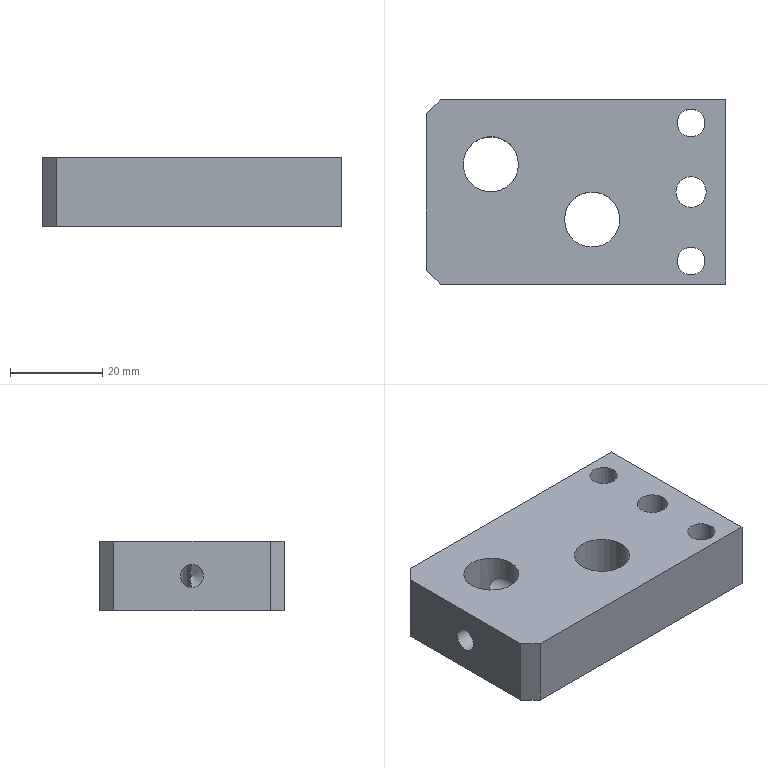Part | NX | features BREP 1 | 1 solid | 20 faces | box 65 x 40 x 15 mm | volume 33188 mm3 | plane 9 | cylinder 9 | cone 2 | commonest cylinder face diameters 5 x3 6 x2 12 x2 6.6 x1 11 x1
STEP:
#1=CARTESIAN_POINT('',(32.5,-20.,0.));
#2=VERTEX_POINT('',#1);
#3=CARTESIAN_POINT('',(32.5,20.,0.));
#4=VERTEX_POINT('',#3);
#5=CARTESIAN_POINT('',(32.5,20.,0.));
#6=DIRECTION('',(0.,1.,0.));
#7=VECTOR('',#6,1000.);
#8=LINE('',#5,#7);
#9=EDGE_CURVE('',#2,#4,#8,.T.);
#10=ORIENTED_EDGE('',*,*,#9,.T.);
#11=CARTESIAN_POINT('',(32.5,20.,15.));
#12=VERTEX_POINT('',#11);
#13=CARTESIAN_POINT('',(32.5,20.,15.));
#14=DIRECTION('',(0.,0.,-1.));
#15=VECTOR('',#14,1000.);
#16=LINE('',#13,#15);
#17=EDGE_CURVE('',#12,#4,#16,.T.);
#18=ORIENTED_EDGE('',*,*,#17,.F.);
#19=CARTESIAN_POINT('',(32.5,-20.,15.));
#20=VERTEX_POINT('',#19);
#21=CARTESIAN_POINT('',(32.5,20.,15.));
#22=DIRECTION('',(0.,1.,0.));
#23=VECTOR('',#22,1000.);
#24=LINE('',#21,#23);
#25=EDGE_CURVE('',#20,#12,#24,.T.);
#26=ORIENTED_EDGE('',*,*,#25,.F.);
#27=CARTESIAN_POINT('',(32.5,-20.,15.));
#28=DIRECTION('',(0.,0.,-1.));
#29=VECTOR('',#28,1000.);
#30=LINE('',#27,#29);
#31=EDGE_CURVE('',#20,#2,#30,.T.);
#32=ORIENTED_EDGE('',*,*,#31,.T.);
#33=EDGE_LOOP('',(#10,#18,#26,#32));
#34=FACE_BOUND('',#33,.T.);
#35=CARTESIAN_POINT('',(32.5,20.,15.));
#36=DIRECTION('',(-1.,0.,0.));
#37=DIRECTION('',(0.,0.,-1.));
#38=AXIS2_PLACEMENT_3D('',#35,#36,#37);
#39=PLANE('',#38);
#40=ADVANCED_FACE('',(#34),#39,.F.);
#41=CARTESIAN_POINT('',(-12.,20.,10.));
#42=VERTEX_POINT('',#41);
#43=CARTESIAN_POINT('',(-12.,20.,7.5));
#44=DIRECTION('',(0.,1.,0.));
#45=DIRECTION('',(0.,0.,1.));
#46=AXIS2_PLACEMENT_3D('',#43,#44,#45);
#47=CIRCLE('',#46,2.5);
#48=EDGE_CURVE('',#42,#42,#47,.T.);
#49=ORIENTED_EDGE('',*,*,#48,.F.);
#50=EDGE_LOOP('',(#49));
#51=FACE_BOUND('',#50,.T.);
#52=CARTESIAN_POINT('',(-29.5,20.,0.));
#53=VERTEX_POINT('',#52);
#54=CARTESIAN_POINT('',(-32.5,20.,0.));
#55=DIRECTION('',(-1.,0.,0.));
#56=VECTOR('',#55,1000.);
#57=LINE('',#54,#56);
#58=EDGE_CURVE('',#4,#53,#57,.T.);
#59=ORIENTED_EDGE('',*,*,#58,.T.);
#60=CARTESIAN_POINT('',(-29.5,20.,15.));
#61=VERTEX_POINT('',#60);
#62=CARTESIAN_POINT('',(-29.5,20.,15.));
#63=DIRECTION('',(0.,0.,1.));
#64=VECTOR('',#63,1000.);
#65=LINE('',#62,#64);
#66=EDGE_CURVE('',#53,#61,#65,.T.);
#67=ORIENTED_EDGE('',*,*,#66,.T.);
#68=CARTESIAN_POINT('',(-32.5,20.,15.));
#69=DIRECTION('',(-1.,0.,0.));
#70=VECTOR('',#69,1000.);
#71=LINE('',#68,#70);
#72=EDGE_CURVE('',#12,#61,#71,.T.);
#73=ORIENTED_EDGE('',*,*,#72,.F.);
#74=ORIENTED_EDGE('',*,*,#17,.T.);
#75=EDGE_LOOP('',(#59,#67,#73,#74));
#76=FACE_BOUND('',#75,.T.);
#77=CARTESIAN_POINT('',(-32.5,20.,15.));
#78=DIRECTION('',(0.,-1.,0.));
#79=DIRECTION('',(0.,0.,1.));
#80=AXIS2_PLACEMENT_3D('',#77,#78,#79);
#81=PLANE('',#80);
#82=ADVANCED_FACE('',(#51,#76),#81,.F.);
#83=CARTESIAN_POINT('',(-32.5,0.,10.));
#84=VERTEX_POINT('',#83);
#85=CARTESIAN_POINT('',(-32.5,0.,7.5));
#86=DIRECTION('',(-1.,0.,0.));
#87=DIRECTION('',(0.,0.,1.));
#88=AXIS2_PLACEMENT_3D('',#85,#86,#87);
#89=CIRCLE('',#88,2.5);
#90=EDGE_CURVE('',#84,#84,#89,.T.);
#91=ORIENTED_EDGE('',*,*,#90,.F.);
#92=EDGE_LOOP('',(#91));
#93=FACE_BOUND('',#92,.T.);
#94=CARTESIAN_POINT('',(-32.5,17.,15.));
#95=VERTEX_POINT('',#94);
#96=CARTESIAN_POINT('',(-32.5,-17.,15.));
#97=VERTEX_POINT('',#96);
#98=CARTESIAN_POINT('',(-32.5,20.,15.));
#99=DIRECTION('',(0.,-1.,0.));
#100=VECTOR('',#99,1000.);
#101=LINE('',#98,#100);
#102=EDGE_CURVE('',#95,#97,#101,.T.);
#103=ORIENTED_EDGE('',*,*,#102,.F.);
#104=CARTESIAN_POINT('',(-32.5,17.,0.));
#105=VERTEX_POINT('',#104);
#106=CARTESIAN_POINT('',(-32.5,17.,15.));
#107=DIRECTION('',(0.,0.,-1.));
#108=VECTOR('',#107,1000.);
#109=LINE('',#106,#108);
#110=EDGE_CURVE('',#95,#105,#109,.T.);
#111=ORIENTED_EDGE('',*,*,#110,.T.);
#112=CARTESIAN_POINT('',(-32.5,-17.,0.));
#113=VERTEX_POINT('',#112);
#114=CARTESIAN_POINT('',(-32.5,20.,0.));
#115=DIRECTION('',(0.,-1.,0.));
#116=VECTOR('',#115,1000.);
#117=LINE('',#114,#116);
#118=EDGE_CURVE('',#105,#113,#117,.T.);
#119=ORIENTED_EDGE('',*,*,#118,.T.);
#120=CARTESIAN_POINT('',(-32.5,-17.,15.));
#121=DIRECTION('',(0.,0.,1.));
#122=VECTOR('',#121,1000.);
#123=LINE('',#120,#122);
#124=EDGE_CURVE('',#113,#97,#123,.T.);
#125=ORIENTED_EDGE('',*,*,#124,.T.);
#126=EDGE_LOOP('',(#103,#111,#119,#125));
#127=FACE_BOUND('',#126,.T.);
#128=CARTESIAN_POINT('',(-32.5,20.,15.));
#129=DIRECTION('',(1.,0.,0.));
#130=DIRECTION('',(0.,-1.,0.));
#131=AXIS2_PLACEMENT_3D('',#128,#129,#130);
#132=PLANE('',#131);
#133=ADVANCED_FACE('',(#93,#127),#132,.F.);
#134=CARTESIAN_POINT('',(-29.5,-20.,15.));
#135=VERTEX_POINT('',#134);
#136=CARTESIAN_POINT('',(-32.5,-20.,15.));
#137=DIRECTION('',(1.,0.,0.));
#138=VECTOR('',#137,1000.);
#139=LINE('',#136,#138);
#140=EDGE_CURVE('',#135,#20,#139,.T.);
#141=ORIENTED_EDGE('',*,*,#140,.F.);
#142=CARTESIAN_POINT('',(-29.5,-20.,0.));
#143=VERTEX_POINT('',#142);
#144=CARTESIAN_POINT('',(-29.5,-20.,15.));
#145=DIRECTION('',(0.,0.,-1.));
#146=VECTOR('',#145,1000.);
#147=LINE('',#144,#146);
#148=EDGE_CURVE('',#135,#143,#147,.T.);
#149=ORIENTED_EDGE('',*,*,#148,.T.);
#150=CARTESIAN_POINT('',(-32.5,-20.,0.));
#151=DIRECTION('',(1.,0.,0.));
#152=VECTOR('',#151,1000.);
#153=LINE('',#150,#152);
#154=EDGE_CURVE('',#143,#2,#153,.T.);
#155=ORIENTED_EDGE('',*,*,#154,.T.);
#156=ORIENTED_EDGE('',*,*,#31,.F.);
#157=EDGE_LOOP('',(#141,#149,#155,#156));
#158=FACE_BOUND('',#157,.T.);
#159=CARTESIAN_POINT('',(-32.5,-20.,15.));
#160=DIRECTION('',(0.,1.,0.));
#161=DIRECTION('',(0.,0.,-1.));
#162=AXIS2_PLACEMENT_3D('',#159,#160,#161);
#163=PLANE('',#162);
#164=ADVANCED_FACE('',(#158),#163,.F.);
#165=CARTESIAN_POINT('',(21.7,0.,15.));
#166=VERTEX_POINT('',#165);
#167=CARTESIAN_POINT('',(25.,0.,15.));
#168=DIRECTION('',(0.,0.,-1.));
#169=DIRECTION('',(-1.,0.,0.));
#170=AXIS2_PLACEMENT_3D('',#167,#168,#169);
#171=CIRCLE('',#170,3.3);
#172=EDGE_CURVE('',#166,#166,#171,.T.);
#173=ORIENTED_EDGE('',*,*,#172,.T.);
#174=EDGE_LOOP('',(#173));
#175=FACE_BOUND('',#174,.T.);
#176=CARTESIAN_POINT('',(28.,-15.,15.));
#177=VERTEX_POINT('',#176);
#178=CARTESIAN_POINT('',(25.,-15.,15.));
#179=DIRECTION('',(0.,0.,1.));
#180=DIRECTION('',(1.,0.,0.));
#181=AXIS2_PLACEMENT_3D('',#178,#179,#180);
#182=CIRCLE('',#181,3.);
#183=EDGE_CURVE('',#177,#177,#182,.T.);
#184=ORIENTED_EDGE('',*,*,#183,.F.);
#185=EDGE_LOOP('',(#184));
#186=FACE_BOUND('',#185,.T.);
#187=CARTESIAN_POINT('',(28.,15.,15.));
#188=VERTEX_POINT('',#187);
#189=CARTESIAN_POINT('',(25.,15.,15.));
#190=DIRECTION('',(0.,0.,1.));
#191=DIRECTION('',(1.,0.,0.));
#192=AXIS2_PLACEMENT_3D('',#189,#190,#191);
#193=CIRCLE('',#192,3.);
#194=EDGE_CURVE('',#188,#188,#193,.T.);
#195=ORIENTED_EDGE('',*,*,#194,.F.);
#196=EDGE_LOOP('',(#195));
#197=FACE_BOUND('',#196,.T.);
#198=CARTESIAN_POINT('',(-12.5,6.,15.));
#199=VERTEX_POINT('',#198);
#200=CARTESIAN_POINT('',(-18.5,6.,15.));
#201=DIRECTION('',(0.,0.,1.));
#202=DIRECTION('',(1.,0.,0.));
#203=AXIS2_PLACEMENT_3D('',#200,#201,#202);
#204=CIRCLE('',#203,6.);
#205=EDGE_CURVE('',#199,#199,#204,.T.);
#206=ORIENTED_EDGE('',*,*,#205,.F.);
#207=EDGE_LOOP('',(#206));
#208=FACE_BOUND('',#207,.T.);
#209=CARTESIAN_POINT('',(9.5,-6.,15.));
#210=VERTEX_POINT('',#209);
#211=CARTESIAN_POINT('',(3.5,-6.,15.));
#212=DIRECTION('',(0.,0.,1.));
#213=DIRECTION('',(1.,0.,0.));
#214=AXIS2_PLACEMENT_3D('',#211,#212,#213);
#215=CIRCLE('',#214,6.);
#216=EDGE_CURVE('',#210,#210,#215,.T.);
#217=ORIENTED_EDGE('',*,*,#216,.F.);
#218=EDGE_LOOP('',(#217));
#219=FACE_BOUND('',#218,.T.);
#220=ORIENTED_EDGE('',*,*,#72,.T.);
#221=CARTESIAN_POINT('',(-24.75,24.75,15.));
#222=DIRECTION('',(-0.7071,-0.7071,0.));
#223=VECTOR('',#222,1000.);
#224=LINE('',#221,#223);
#225=EDGE_CURVE('',#61,#95,#224,.T.);
#226=ORIENTED_EDGE('',*,*,#225,.T.);
#227=ORIENTED_EDGE('',*,*,#102,.T.);
#228=CARTESIAN_POINT('',(-24.75,-24.75,15.));
#229=DIRECTION('',(0.7071,-0.7071,0.));
#230=VECTOR('',#229,1000.);
#231=LINE('',#228,#230);
#232=EDGE_CURVE('',#97,#135,#231,.T.);
#233=ORIENTED_EDGE('',*,*,#232,.T.);
#234=ORIENTED_EDGE('',*,*,#140,.T.);
#235=ORIENTED_EDGE('',*,*,#25,.T.);
#236=EDGE_LOOP('',(#220,#226,#227,#233,#234,#235));
#237=FACE_BOUND('',#236,.T.);
#238=CARTESIAN_POINT('',(0.,0.,15.));
#239=DIRECTION('',(0.,0.,1.));
#240=DIRECTION('',(-1.,0.,0.));
#241=AXIS2_PLACEMENT_3D('',#238,#239,#240);
#242=PLANE('',#241);
#243=ADVANCED_FACE('',(#175,#186,#197,#208,#219,#237),#242,.T.);
#244=CARTESIAN_POINT('',(19.5,0.,0.));
#245=VERTEX_POINT('',#244);
#246=CARTESIAN_POINT('',(25.,0.,0.));
#247=DIRECTION('',(0.,0.,-1.));
#248=DIRECTION('',(-1.,0.,0.));
#249=AXIS2_PLACEMENT_3D('',#246,#247,#248);
#250=CIRCLE('',#249,5.5);
#251=EDGE_CURVE('',#245,#245,#250,.T.);
#252=ORIENTED_EDGE('',*,*,#251,.F.);
#253=EDGE_LOOP('',(#252));
#254=FACE_BOUND('',#253,.T.);
#255=CARTESIAN_POINT('',(28.,-15.,0.));
#256=VERTEX_POINT('',#255);
#257=CARTESIAN_POINT('',(25.,-15.,0.));
#258=DIRECTION('',(0.,0.,1.));
#259=DIRECTION('',(1.,0.,0.));
#260=AXIS2_PLACEMENT_3D('',#257,#258,#259);
#261=CIRCLE('',#260,3.);
#262=EDGE_CURVE('',#256,#256,#261,.T.);
#263=ORIENTED_EDGE('',*,*,#262,.T.);
#264=EDGE_LOOP('',(#263));
#265=FACE_BOUND('',#264,.T.);
#266=CARTESIAN_POINT('',(28.,15.,0.));
#267=VERTEX_POINT('',#266);
#268=CARTESIAN_POINT('',(25.,15.,0.));
#269=DIRECTION('',(0.,0.,1.));
#270=DIRECTION('',(1.,0.,0.));
#271=AXIS2_PLACEMENT_3D('',#268,#269,#270);
#272=CIRCLE('',#271,3.);
#273=EDGE_CURVE('',#267,#267,#272,.T.);
#274=ORIENTED_EDGE('',*,*,#273,.T.);
#275=EDGE_LOOP('',(#274));
#276=FACE_BOUND('',#275,.T.);
#277=CARTESIAN_POINT('',(-12.5,6.,0.));
#278=VERTEX_POINT('',#277);
#279=CARTESIAN_POINT('',(-18.5,6.,0.));
#280=DIRECTION('',(0.,0.,1.));
#281=DIRECTION('',(1.,0.,0.));
#282=AXIS2_PLACEMENT_3D('',#279,#280,#281);
#283=CIRCLE('',#282,6.);
#284=EDGE_CURVE('',#278,#278,#283,.T.);
#285=ORIENTED_EDGE('',*,*,#284,.T.);
#286=EDGE_LOOP('',(#285));
#287=FACE_BOUND('',#286,.T.);
#288=CARTESIAN_POINT('',(9.5,-6.,0.));
#289=VERTEX_POINT('',#288);
#290=CARTESIAN_POINT('',(3.5,-6.,0.));
#291=DIRECTION('',(0.,0.,1.));
#292=DIRECTION('',(1.,0.,0.));
#293=AXIS2_PLACEMENT_3D('',#290,#291,#292);
#294=CIRCLE('',#293,6.);
#295=EDGE_CURVE('',#289,#289,#294,.T.);
#296=ORIENTED_EDGE('',*,*,#295,.T.);
#297=EDGE_LOOP('',(#296));
#298=FACE_BOUND('',#297,.T.);
#299=ORIENTED_EDGE('',*,*,#118,.F.);
#300=CARTESIAN_POINT('',(-32.5,17.,0.));
#301=DIRECTION('',(0.7071,0.7071,0.));
#302=VECTOR('',#301,1000.);
#303=LINE('',#300,#302);
#304=EDGE_CURVE('',#105,#53,#303,.T.);
#305=ORIENTED_EDGE('',*,*,#304,.T.);
#306=ORIENTED_EDGE('',*,*,#58,.F.);
#307=ORIENTED_EDGE('',*,*,#9,.F.);
#308=ORIENTED_EDGE('',*,*,#154,.F.);
#309=CARTESIAN_POINT('',(-29.5,-20.,0.));
#310=DIRECTION('',(-0.7071,0.7071,0.));
#311=VECTOR('',#310,1000.);
#312=LINE('',#309,#311);
#313=EDGE_CURVE('',#143,#113,#312,.T.);
#314=ORIENTED_EDGE('',*,*,#313,.T.);
#315=EDGE_LOOP('',(#299,#305,#306,#307,#308,#314));
#316=FACE_BOUND('',#315,.T.);
#317=CARTESIAN_POINT('',(0.,0.,0.));
#318=DIRECTION('',(0.,0.,1.));
#319=DIRECTION('',(-1.,0.,0.));
#320=AXIS2_PLACEMENT_3D('',#317,#318,#319);
#321=PLANE('',#320);
#322=ADVANCED_FACE('',(#254,#265,#276,#287,#298,#316),#321,.F.);
#323=ORIENTED_EDGE('',*,*,#295,.F.);
#324=EDGE_LOOP('',(#323));
#325=FACE_BOUND('',#324,.T.);
#326=ORIENTED_EDGE('',*,*,#216,.T.);
#327=EDGE_LOOP('',(#326));
#328=FACE_BOUND('',#327,.T.);
#329=CARTESIAN_POINT('',(3.5,-6.,15.));
#330=DIRECTION('',(0.,0.,1.));
#331=DIRECTION('',(-1.,0.,0.));
#332=AXIS2_PLACEMENT_3D('',#329,#330,#331);
#333=CYLINDRICAL_SURFACE('',#332,6.);
#334=ADVANCED_FACE('',(#325,#328),#333,.F.);
#335=CARTESIAN_POINT('',(-12.584,5.,9.931));
#336=VERTEX_POINT('',#335);
#337=CARTESIAN_POINT('',(-12.584,5.,5.069));
#338=VERTEX_POINT('',#337);
#339=CARTESIAN_POINT('',(-12.584,5.,9.931));
#340=CARTESIAN_POINT('',(-12.621,4.78,9.545));
#341=CARTESIAN_POINT('',(-12.719,4.353,8.787));
#342=CARTESIAN_POINT('',(-12.904,3.829,7.497));
#343=CARTESIAN_POINT('',(-12.718,4.355,6.211));
#344=CARTESIAN_POINT('',(-12.621,4.781,5.454));
#345=CARTESIAN_POINT('',(-12.584,5.,5.069));
#346=B_SPLINE_CURVE_WITH_KNOTS('',3,(#339,#340,#341,#342,#343,#344,#345),.UNSPECIFIED.,.F.,.F.,(4,1,1,1,4),(0.,0.001335,0.002669,0.004004,0.005339),.UNSPECIFIED.);
#347=EDGE_CURVE('',#336,#338,#346,.T.);
#348=ORIENTED_EDGE('',*,*,#347,.T.);
#349=CARTESIAN_POINT('',(-12.584,5.,5.069));
#350=CARTESIAN_POINT('',(-12.483,5.598,5.045));
#351=CARTESIAN_POINT('',(-12.466,6.805,5.043));
#352=CARTESIAN_POINT('',(-12.961,8.547,5.154));
#353=CARTESIAN_POINT('',(-13.981,10.042,5.725));
#354=CARTESIAN_POINT('',(-14.757,10.685,7.487));
#355=CARTESIAN_POINT('',(-13.992,10.053,9.265));
#356=CARTESIAN_POINT('',(-12.971,8.568,9.843));
#357=CARTESIAN_POINT('',(-12.466,6.82,9.957));
#358=CARTESIAN_POINT('',(-12.483,5.598,9.955));
#359=CARTESIAN_POINT('',(-12.584,5.,9.931));
#360=B_SPLINE_CURVE_WITH_KNOTS('',3,(#349,#350,#351,#352,#353,#354,#355,#356,#357,#358,#359),.UNSPECIFIED.,.F.,.F.,(4,1,1,1,1,1,1,1,4),(0.,0.001794,0.003588,0.005381,0.007175,0.008969,0.01076,0.01256,0.01435),.UNSPECIFIED.);
#361=EDGE_CURVE('',#338,#336,#360,.T.);
#362=ORIENTED_EDGE('',*,*,#361,.T.);
#363=EDGE_LOOP('',(#348,#362));
#364=FACE_BOUND('',#363,.T.);
#365=CARTESIAN_POINT('',(-17.5,0.08392,5.001));
#366=VERTEX_POINT('',#365);
#367=CARTESIAN_POINT('',(-17.5,0.08392,9.999));
#368=VERTEX_POINT('',#367);
#369=CARTESIAN_POINT('',(-17.5,0.08392,5.001));
#370=CARTESIAN_POINT('',(-17.258,0.1249,5.406));
#371=CARTESIAN_POINT('',(-16.894,0.21,6.015));
#372=CARTESIAN_POINT('',(-16.442,0.3603,6.82));
#373=CARTESIAN_POINT('',(-16.166,0.4718,7.506));
#374=CARTESIAN_POINT('',(-16.448,0.3584,8.187));
#375=CARTESIAN_POINT('',(-16.896,0.2095,8.99));
#376=CARTESIAN_POINT('',(-17.259,0.1247,9.595));
#377=CARTESIAN_POINT('',(-17.5,0.08392,9.999));
#378=B_SPLINE_CURVE_WITH_KNOTS('',3,(#369,#370,#371,#372,#373,#374,#375,#376,#377),.UNSPECIFIED.,.F.,.F.,(4,1,1,1,1,1,4),(0.,0.00142,0.002129,0.002839,0.003549,0.004259,0.005678),.UNSPECIFIED.);
#379=EDGE_CURVE('',#366,#368,#378,.T.);
#380=ORIENTED_EDGE('',*,*,#379,.T.);
#381=CARTESIAN_POINT('',(-17.5,0.08392,9.999));
#382=CARTESIAN_POINT('',(-18.156,-0.02704,10.002));
#383=CARTESIAN_POINT('',(-19.485,-0.02533,10.002));
#384=CARTESIAN_POINT('',(-21.382,0.6017,9.983));
#385=CARTESIAN_POINT('',(-22.962,1.871,9.453));
#386=CARTESIAN_POINT('',(-23.576,2.81,7.515));
#387=CARTESIAN_POINT('',(-22.974,1.887,5.559));
#388=CARTESIAN_POINT('',(-21.4,0.6113,5.019));
#389=CARTESIAN_POINT('',(-19.499,-0.0247,4.998));
#390=CARTESIAN_POINT('',(-18.157,-0.02714,4.998));
#391=CARTESIAN_POINT('',(-17.5,0.08392,5.001));
#392=B_SPLINE_CURVE_WITH_KNOTS('',3,(#381,#382,#383,#384,#385,#386,#387,#388,#389,#390,#391),.UNSPECIFIED.,.F.,.F.,(4,1,1,1,1,1,1,1,4),(0.,0.001969,0.003938,0.005907,0.007876,0.009845,0.01181,0.01378,0.01575),.UNSPECIFIED.);
#393=EDGE_CURVE('',#368,#366,#392,.T.);
#394=ORIENTED_EDGE('',*,*,#393,.T.);
#395=EDGE_LOOP('',(#380,#394));
#396=FACE_BOUND('',#395,.T.);
#397=ORIENTED_EDGE('',*,*,#284,.F.);
#398=EDGE_LOOP('',(#397));
#399=FACE_BOUND('',#398,.T.);
#400=ORIENTED_EDGE('',*,*,#205,.T.);
#401=EDGE_LOOP('',(#400));
#402=FACE_BOUND('',#401,.T.);
#403=CARTESIAN_POINT('',(-18.5,6.,15.));
#404=DIRECTION('',(0.,0.,1.));
#405=DIRECTION('',(-1.,0.,0.));
#406=AXIS2_PLACEMENT_3D('',#403,#404,#405);
#407=CYLINDRICAL_SURFACE('',#406,6.);
#408=ADVANCED_FACE('',(#364,#396,#399,#402),#407,.F.);
#409=ORIENTED_EDGE('',*,*,#273,.F.);
#410=EDGE_LOOP('',(#409));
#411=FACE_BOUND('',#410,.T.);
#412=ORIENTED_EDGE('',*,*,#194,.T.);
#413=EDGE_LOOP('',(#412));
#414=FACE_BOUND('',#413,.T.);
#415=CARTESIAN_POINT('',(25.,15.,15.));
#416=DIRECTION('',(0.,0.,1.));
#417=DIRECTION('',(-1.,0.,0.));
#418=AXIS2_PLACEMENT_3D('',#415,#416,#417);
#419=CYLINDRICAL_SURFACE('',#418,3.);
#420=ADVANCED_FACE('',(#411,#414),#419,.F.);
#421=ORIENTED_EDGE('',*,*,#262,.F.);
#422=EDGE_LOOP('',(#421));
#423=FACE_BOUND('',#422,.T.);
#424=ORIENTED_EDGE('',*,*,#183,.T.);
#425=EDGE_LOOP('',(#424));
#426=FACE_BOUND('',#425,.T.);
#427=CARTESIAN_POINT('',(25.,-15.,15.));
#428=DIRECTION('',(0.,0.,1.));
#429=DIRECTION('',(-1.,0.,0.));
#430=AXIS2_PLACEMENT_3D('',#427,#428,#429);
#431=CYLINDRICAL_SURFACE('',#430,3.);
#432=ADVANCED_FACE('',(#423,#426),#431,.F.);
#433=ORIENTED_EDGE('',*,*,#172,.F.);
#434=EDGE_LOOP('',(#433));
#435=FACE_BOUND('',#434,.T.);
#436=CARTESIAN_POINT('',(21.7,0.,6.4));
#437=VERTEX_POINT('',#436);
#438=CARTESIAN_POINT('',(25.,0.,6.4));
#439=DIRECTION('',(0.,0.,-1.));
#440=DIRECTION('',(-1.,0.,0.));
#441=AXIS2_PLACEMENT_3D('',#438,#439,#440);
#442=CIRCLE('',#441,3.3);
#443=EDGE_CURVE('',#437,#437,#442,.T.);
#444=ORIENTED_EDGE('',*,*,#443,.T.);
#445=EDGE_LOOP('',(#444));
#446=FACE_BOUND('',#445,.T.);
#447=CARTESIAN_POINT('',(25.,0.,0.));
#448=DIRECTION('',(0.,0.,-1.));
#449=DIRECTION('',(1.,0.,0.));
#450=AXIS2_PLACEMENT_3D('',#447,#448,#449);
#451=CYLINDRICAL_SURFACE('',#450,3.3);
#452=ADVANCED_FACE('',(#435,#446),#451,.F.);
#453=ORIENTED_EDGE('',*,*,#443,.F.);
#454=EDGE_LOOP('',(#453));
#455=FACE_BOUND('',#454,.T.);
#456=CARTESIAN_POINT('',(19.5,0.,6.4));
#457=VERTEX_POINT('',#456);
#458=CARTESIAN_POINT('',(25.,0.,6.4));
#459=DIRECTION('',(0.,0.,-1.));
#460=DIRECTION('',(-1.,0.,0.));
#461=AXIS2_PLACEMENT_3D('',#458,#459,#460);
#462=CIRCLE('',#461,5.5);
#463=EDGE_CURVE('',#457,#457,#462,.T.);
#464=ORIENTED_EDGE('',*,*,#463,.T.);
#465=EDGE_LOOP('',(#464));
#466=FACE_BOUND('',#465,.T.);
#467=CARTESIAN_POINT('',(28.3,0.,6.4));
#468=DIRECTION('',(0.,0.,1.));
#469=DIRECTION('',(-1.,0.,0.));
#470=AXIS2_PLACEMENT_3D('',#467,#468,#469);
#471=PLANE('',#470);
#472=ADVANCED_FACE('',(#455,#466),#471,.F.);
#473=ORIENTED_EDGE('',*,*,#463,.F.);
#474=EDGE_LOOP('',(#473));
#475=FACE_BOUND('',#474,.T.);
#476=ORIENTED_EDGE('',*,*,#251,.T.);
#477=EDGE_LOOP('',(#476));
#478=FACE_BOUND('',#477,.T.);
#479=CARTESIAN_POINT('',(25.,0.,0.));
#480=DIRECTION('',(0.,0.,-1.));
#481=DIRECTION('',(1.,0.,0.));
#482=AXIS2_PLACEMENT_3D('',#479,#480,#481);
#483=CYLINDRICAL_SURFACE('',#482,5.5);
#484=ADVANCED_FACE('',(#475,#478),#483,.F.);
#485=ORIENTED_EDGE('',*,*,#225,.F.);
#486=ORIENTED_EDGE('',*,*,#66,.F.);
#487=ORIENTED_EDGE('',*,*,#304,.F.);
#488=ORIENTED_EDGE('',*,*,#110,.F.);
#489=EDGE_LOOP('',(#485,#486,#487,#488));
#490=FACE_BOUND('',#489,.T.);
#491=CARTESIAN_POINT('',(-32.5,17.,15.));
#492=DIRECTION('',(0.7071,-0.7071,0.));
#493=DIRECTION('',(0.,0.,1.));
#494=AXIS2_PLACEMENT_3D('',#491,#492,#493);
#495=PLANE('',#494);
#496=ADVANCED_FACE('',(#490),#495,.F.);
#497=ORIENTED_EDGE('',*,*,#232,.F.);
#498=ORIENTED_EDGE('',*,*,#124,.F.);
#499=ORIENTED_EDGE('',*,*,#313,.F.);
#500=ORIENTED_EDGE('',*,*,#148,.F.);
#501=EDGE_LOOP('',(#497,#498,#499,#500));
#502=FACE_BOUND('',#501,.T.);
#503=CARTESIAN_POINT('',(-29.5,-20.,15.));
#504=DIRECTION('',(0.7071,0.7071,0.));
#505=DIRECTION('',(0.,0.,1.));
#506=AXIS2_PLACEMENT_3D('',#503,#504,#505);
#507=PLANE('',#506);
#508=ADVANCED_FACE('',(#502),#507,.F.);
#509=ORIENTED_EDGE('',*,*,#90,.T.);
#510=EDGE_LOOP('',(#509));
#511=FACE_BOUND('',#510,.T.);
#512=CARTESIAN_POINT('',(-17.5,0.,7.5));
#513=DIRECTION('',(-1.,0.,0.));
#514=DIRECTION('',(0.,0.,1.));
#515=AXIS2_PLACEMENT_3D('',#512,#513,#514);
#516=CIRCLE('',#515,2.5);
#517=EDGE_CURVE('',#366,#368,#516,.T.);
#518=ORIENTED_EDGE('',*,*,#517,.F.);
#519=ORIENTED_EDGE('',*,*,#393,.F.);
#520=EDGE_LOOP('',(#518,#519));
#521=FACE_BOUND('',#520,.T.);
#522=CARTESIAN_POINT('',(-32.5,0.,7.5));
#523=DIRECTION('',(-1.,0.,0.));
#524=DIRECTION('',(0.,0.,-1.));
#525=AXIS2_PLACEMENT_3D('',#522,#523,#524);
#526=CYLINDRICAL_SURFACE('',#525,2.5);
#527=ADVANCED_FACE('',(#511,#521),#526,.F.);
#528=ORIENTED_EDGE('',*,*,#517,.T.);
#529=ORIENTED_EDGE('',*,*,#379,.F.);
#530=EDGE_LOOP('',(#528,#529));
#531=FACE_BOUND('',#530,.T.);
#532=CARTESIAN_POINT('',(-17.5,0.,7.5));
#533=DIRECTION('',(-1.,0.,0.));
#534=DIRECTION('',(0.,0.,-1.));
#535=AXIS2_PLACEMENT_3D('',#532,#533,#534);
#536=CONICAL_SURFACE('',#535,2.5,1.03);
#537=ADVANCED_FACE('',(#531),#536,.F.);
#538=ORIENTED_EDGE('',*,*,#48,.T.);
#539=EDGE_LOOP('',(#538));
#540=FACE_BOUND('',#539,.T.);
#541=CARTESIAN_POINT('',(-12.,5.,7.5));
#542=DIRECTION('',(0.,1.,0.));
#543=DIRECTION('',(0.,0.,1.));
#544=AXIS2_PLACEMENT_3D('',#541,#542,#543);
#545=CIRCLE('',#544,2.5);
#546=EDGE_CURVE('',#336,#338,#545,.T.);
#547=ORIENTED_EDGE('',*,*,#546,.F.);
#548=ORIENTED_EDGE('',*,*,#361,.F.);
#549=EDGE_LOOP('',(#547,#548));
#550=FACE_BOUND('',#549,.T.);
#551=CARTESIAN_POINT('',(-12.,20.,7.5));
#552=DIRECTION('',(0.,1.,0.));
#553=DIRECTION('',(0.,0.,-1.));
#554=AXIS2_PLACEMENT_3D('',#551,#552,#553);
#555=CYLINDRICAL_SURFACE('',#554,2.5);
#556=ADVANCED_FACE('',(#540,#550),#555,.F.);
#557=ORIENTED_EDGE('',*,*,#546,.T.);
#558=ORIENTED_EDGE('',*,*,#347,.F.);
#559=EDGE_LOOP('',(#557,#558));
#560=FACE_BOUND('',#559,.T.);
#561=CARTESIAN_POINT('',(-12.,5.,7.5));
#562=DIRECTION('',(0.,1.,0.));
#563=DIRECTION('',(0.,0.,-1.));
#564=AXIS2_PLACEMENT_3D('',#561,#562,#563);
#565=CONICAL_SURFACE('',#564,2.5,1.03);
#566=ADVANCED_FACE('',(#560),#565,.F.);
#567=CLOSED_SHELL('',(#40,#82,#133,#164,#243,#322,#334,#408,#420,#432,#452,#472,#484,#496,#508,#527,#537,#556,#566));
#568=MANIFOLD_SOLID_BREP('',#567);
#569=(LENGTH_UNIT()NAMED_UNIT(*)SI_UNIT(.MILLI.,.METRE.));
#570=UNCERTAINTY_MEASURE_WITH_UNIT(LENGTH_MEASURE(0.0508),#569,'','');
#571=(NAMED_UNIT(*)PLANE_ANGLE_UNIT()SI_UNIT($,.RADIAN.));
#572=(NAMED_UNIT(*)SI_UNIT($,.STERADIAN.)SOLID_ANGLE_UNIT());
#573=(GEOMETRIC_REPRESENTATION_CONTEXT(3)GLOBAL_UNCERTAINTY_ASSIGNED_CONTEXT((#570))GLOBAL_UNIT_ASSIGNED_CONTEXT((#569,#571,#572))REPRESENTATION_CONTEXT('',''));
#574=ADVANCED_BREP_SHAPE_REPRESENTATION('',(#568),#573);